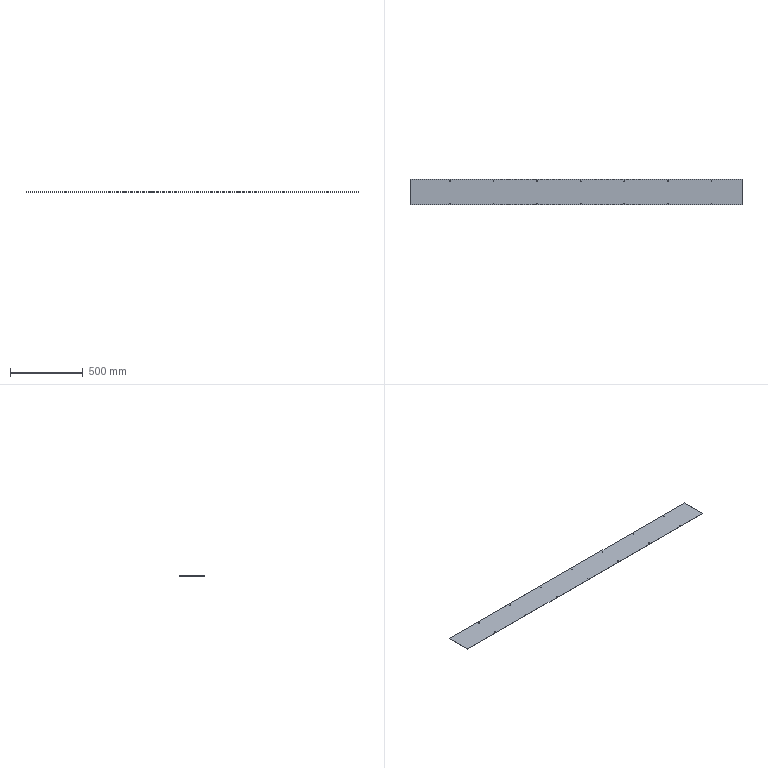Part | STEP file | SX-S21 | 1 solid | 34 faces | box 2285 x 177.5 x 1.2 mm | volume 486320 mm3 | cylinder 28 | plane 6 | commonest cylinder face diameters 5.4 x28